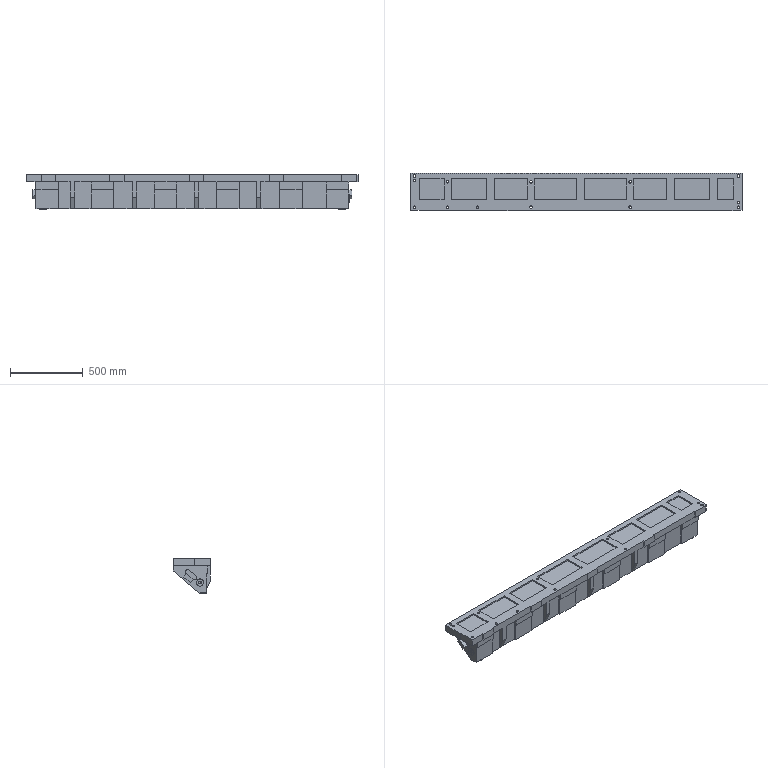Part | NX | features solid 2 | 1 solid | 257 faces | box 2288 x 260.409 x 240 mm | volume 59548439 mm3 | plane 213 | cylinder 39 | cone 5 | commonest cylinder face diameters 17 x11 26 x10 20 x6 50 x6 32 x4 16 x2